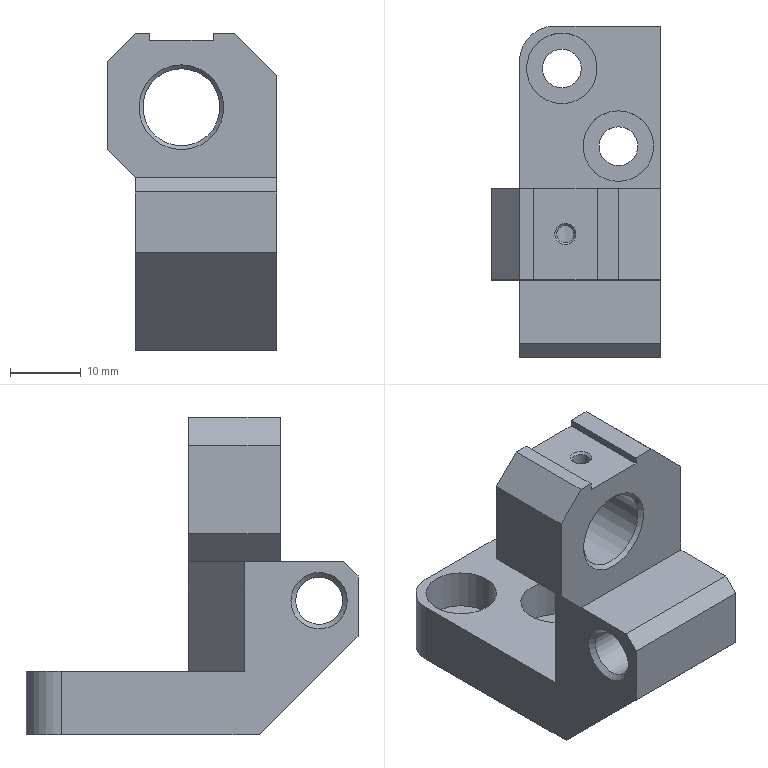Part | STEP file | 1 solid | 37 faces | box 24 x 47 x 45 mm | volume 16099 mm3 | plane 24 | cylinder 8 | cone 5 | commonest cylinder face diameters 10 x3 5.5 x2 2.459 x1 6.647 x1 10.917 x1